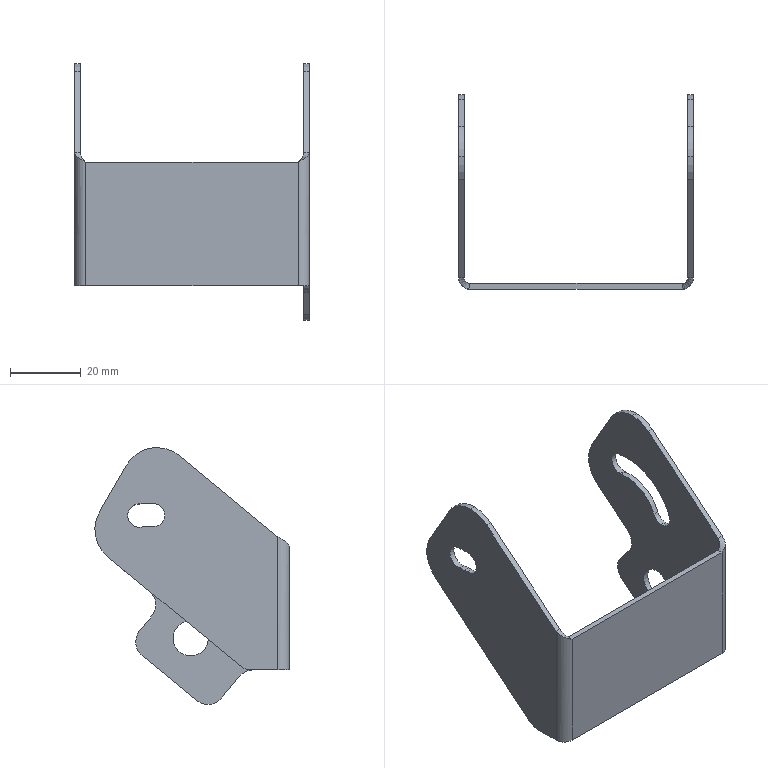Part | SolidWorks | features ICE 5, Fillet 1, FlatPattern 1, SMBaseFlange 1, SheetMetal 1, UnFold 1 | 1 solid | 53 faces | box 66.4 x 55.014 x 72.708 mm | volume 10422 mm3 | cylinder 30 | plane 21 | spline 2 | commonest cylinder face diameters 10 x8 6.6 x6 20 x6 23.4 x3 36.6 x3 3.2 x2